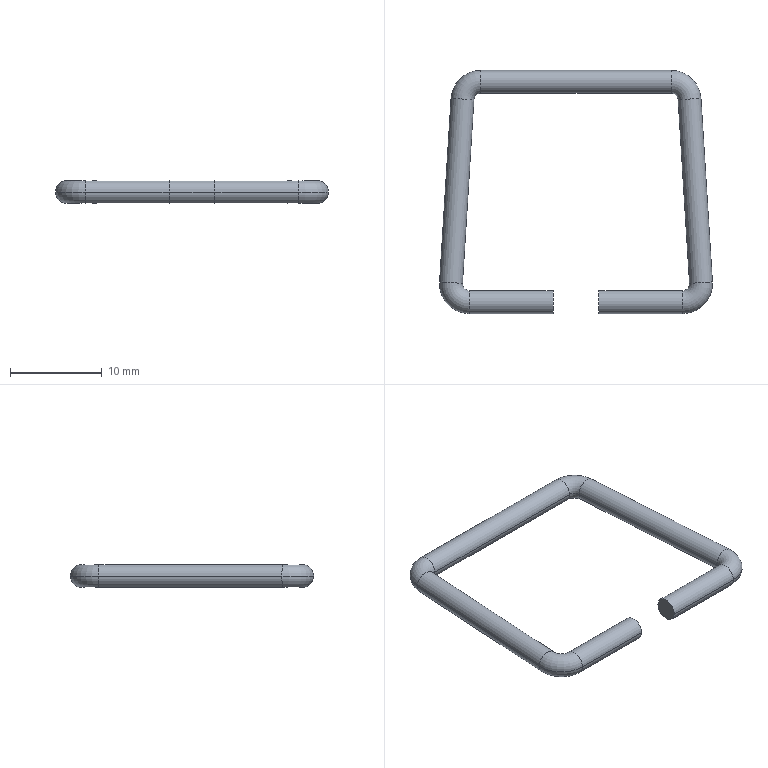Part | SolidWorks | features BaseBody 1 | 1 solid | 20 faces | box 29.742 x 26.5 x 2.5 mm | volume 449.782 mm3 | cylinder 10 | torus 8 | plane 2 | commonest cylinder face diameters 2.5 x10
STEP:
#1=CARTESIAN_POINT('',(11.621,1.25,0.));
#2=VERTEX_POINT('',#1);
#3=CARTESIAN_POINT('',(11.621,-1.25,0.));
#4=VERTEX_POINT('',#3);
#5=CARTESIAN_POINT('',(11.621,0.,0.));
#6=DIRECTION('',(1.,0.,0.));
#7=DIRECTION('',(0.,1.,0.));
#8=AXIS2_PLACEMENT_3D('',#5,#6,#7);
#9=CIRCLE('',#8,1.25);
#10=EDGE_CURVE('',#2,#4,#9,.T.);
#11=ORIENTED_EDGE('',*,*,#10,.T.);
#12=CARTESIAN_POINT('',(14.865,2.203,0.));
#13=VERTEX_POINT('',#12);
#14=CARTESIAN_POINT('',(11.621,2.,0.));
#15=DIRECTION('',(0.,0.,1.));
#16=DIRECTION('',(1.,0.,0.));
#17=AXIS2_PLACEMENT_3D('',#14,#15,#16);
#18=CIRCLE('',#17,3.25);
#19=EDGE_CURVE('',#4,#13,#18,.T.);
#20=ORIENTED_EDGE('',*,*,#19,.T.);
#21=CARTESIAN_POINT('',(12.37,2.047,0.));
#22=VERTEX_POINT('',#21);
#23=CARTESIAN_POINT('',(13.617,2.125,0.));
#24=DIRECTION('',(-0.06238,0.9981,0.));
#25=DIRECTION('',(0.9981,0.06238,0.));
#26=AXIS2_PLACEMENT_3D('',#23,#24,#25);
#27=CIRCLE('',#26,1.25);
#28=EDGE_CURVE('',#22,#13,#27,.T.);
#29=ORIENTED_EDGE('',*,*,#28,.F.);
#30=CARTESIAN_POINT('',(11.621,2.,0.));
#31=DIRECTION('',(0.,0.,1.));
#32=DIRECTION('',(1.,0.,0.));
#33=AXIS2_PLACEMENT_3D('',#30,#31,#32);
#34=CIRCLE('',#33,0.75);
#35=EDGE_CURVE('',#2,#22,#34,.T.);
#36=ORIENTED_EDGE('',*,*,#35,.F.);
#37=EDGE_LOOP('',(#11,#20,#29,#36));
#38=FACE_OUTER_BOUND('',#37,.T.);
#39=CARTESIAN_POINT('',(11.621,2.,0.));
#40=DIRECTION('',(0.,0.,1.));
#41=DIRECTION('',(0.,1.,0.));
#42=AXIS2_PLACEMENT_3D('',#39,#40,#41);
#43=TOROIDAL_SURFACE('',#42,2.,1.25);
#44=ADVANCED_FACE('',(#38),#43,.T.);
#45=CARTESIAN_POINT('',(11.12,22.047,0.));
#46=VERTEX_POINT('',#45);
#47=CARTESIAN_POINT('',(13.615,22.203,0.));
#48=VERTEX_POINT('',#47);
#49=CARTESIAN_POINT('',(12.367,22.125,0.));
#50=DIRECTION('',(-0.06238,0.9981,0.));
#51=DIRECTION('',(-0.9981,-0.06238,0.));
#52=AXIS2_PLACEMENT_3D('',#49,#50,#51);
#53=CIRCLE('',#52,1.25);
#54=EDGE_CURVE('',#46,#48,#53,.T.);
#55=ORIENTED_EDGE('',*,*,#54,.T.);
#56=CARTESIAN_POINT('',(10.371,25.25,0.));
#57=VERTEX_POINT('',#56);
#58=CARTESIAN_POINT('',(10.371,22.,0.));
#59=DIRECTION('',(0.,0.,1.));
#60=DIRECTION('',(1.,0.,0.));
#61=AXIS2_PLACEMENT_3D('',#58,#59,#60);
#62=CIRCLE('',#61,3.25);
#63=EDGE_CURVE('',#48,#57,#62,.T.);
#64=ORIENTED_EDGE('',*,*,#63,.T.);
#65=CARTESIAN_POINT('',(10.371,22.75,0.));
#66=VERTEX_POINT('',#65);
#67=CARTESIAN_POINT('',(10.371,24.,0.));
#68=DIRECTION('',(-1.,0.,0.));
#69=DIRECTION('',(0.,1.,0.));
#70=AXIS2_PLACEMENT_3D('',#67,#68,#69);
#71=CIRCLE('',#70,1.25);
#72=EDGE_CURVE('',#66,#57,#71,.T.);
#73=ORIENTED_EDGE('',*,*,#72,.F.);
#74=CARTESIAN_POINT('',(10.371,22.,0.));
#75=DIRECTION('',(0.,0.,1.));
#76=DIRECTION('',(1.,0.,0.));
#77=AXIS2_PLACEMENT_3D('',#74,#75,#76);
#78=CIRCLE('',#77,0.75);
#79=EDGE_CURVE('',#46,#66,#78,.T.);
#80=ORIENTED_EDGE('',*,*,#79,.F.);
#81=EDGE_LOOP('',(#55,#64,#73,#80));
#82=FACE_OUTER_BOUND('',#81,.T.);
#83=CARTESIAN_POINT('',(10.371,22.,0.));
#84=DIRECTION('',(0.,0.,1.));
#85=DIRECTION('',(-0.9981,-0.06238,0.));
#86=AXIS2_PLACEMENT_3D('',#83,#84,#85);
#87=TOROIDAL_SURFACE('',#86,2.,1.25);
#88=ADVANCED_FACE('',(#82),#87,.T.);
#89=CARTESIAN_POINT('',(-10.371,22.75,0.));
#90=VERTEX_POINT('',#89);
#91=CARTESIAN_POINT('',(-10.371,25.25,0.));
#92=VERTEX_POINT('',#91);
#93=CARTESIAN_POINT('',(-10.371,24.,0.));
#94=DIRECTION('',(-1.,0.,0.));
#95=DIRECTION('',(0.,-1.,0.));
#96=AXIS2_PLACEMENT_3D('',#93,#94,#95);
#97=CIRCLE('',#96,1.25);
#98=EDGE_CURVE('',#90,#92,#97,.T.);
#99=ORIENTED_EDGE('',*,*,#98,.T.);
#100=CARTESIAN_POINT('',(-13.615,22.203,0.));
#101=VERTEX_POINT('',#100);
#102=CARTESIAN_POINT('',(-10.371,22.,0.));
#103=DIRECTION('',(0.,0.,1.));
#104=DIRECTION('',(1.,0.,0.));
#105=AXIS2_PLACEMENT_3D('',#102,#103,#104);
#106=CIRCLE('',#105,3.25);
#107=EDGE_CURVE('',#92,#101,#106,.T.);
#108=ORIENTED_EDGE('',*,*,#107,.T.);
#109=CARTESIAN_POINT('',(-11.12,22.047,0.));
#110=VERTEX_POINT('',#109);
#111=CARTESIAN_POINT('',(-12.367,22.125,0.));
#112=DIRECTION('',(-0.06238,-0.9981,0.));
#113=DIRECTION('',(-0.9981,0.06238,0.));
#114=AXIS2_PLACEMENT_3D('',#111,#112,#113);
#115=CIRCLE('',#114,1.25);
#116=EDGE_CURVE('',#110,#101,#115,.T.);
#117=ORIENTED_EDGE('',*,*,#116,.F.);
#118=CARTESIAN_POINT('',(-10.371,22.,0.));
#119=DIRECTION('',(0.,0.,1.));
#120=DIRECTION('',(1.,0.,0.));
#121=AXIS2_PLACEMENT_3D('',#118,#119,#120);
#122=CIRCLE('',#121,0.75);
#123=EDGE_CURVE('',#90,#110,#122,.T.);
#124=ORIENTED_EDGE('',*,*,#123,.F.);
#125=EDGE_LOOP('',(#99,#108,#117,#124));
#126=FACE_OUTER_BOUND('',#125,.T.);
#127=CARTESIAN_POINT('',(-10.371,22.,0.));
#128=DIRECTION('',(0.,0.,1.));
#129=DIRECTION('',(0.,-1.,0.));
#130=AXIS2_PLACEMENT_3D('',#127,#128,#129);
#131=TOROIDAL_SURFACE('',#130,2.,1.25);
#132=ADVANCED_FACE('',(#126),#131,.T.);
#133=CARTESIAN_POINT('',(-12.37,2.047,0.));
#134=VERTEX_POINT('',#133);
#135=CARTESIAN_POINT('',(-14.865,2.203,0.));
#136=VERTEX_POINT('',#135);
#137=CARTESIAN_POINT('',(-13.617,2.125,0.));
#138=DIRECTION('',(-0.06238,-0.9981,0.));
#139=DIRECTION('',(0.9981,-0.06238,0.));
#140=AXIS2_PLACEMENT_3D('',#137,#138,#139);
#141=CIRCLE('',#140,1.25);
#142=EDGE_CURVE('',#134,#136,#141,.T.);
#143=ORIENTED_EDGE('',*,*,#142,.T.);
#144=CARTESIAN_POINT('',(-11.621,-1.25,0.));
#145=VERTEX_POINT('',#144);
#146=CARTESIAN_POINT('',(-11.621,2.,0.));
#147=DIRECTION('',(0.,0.,1.));
#148=DIRECTION('',(1.,0.,0.));
#149=AXIS2_PLACEMENT_3D('',#146,#147,#148);
#150=CIRCLE('',#149,3.25);
#151=EDGE_CURVE('',#136,#145,#150,.T.);
#152=ORIENTED_EDGE('',*,*,#151,.T.);
#153=CARTESIAN_POINT('',(-11.621,1.25,0.));
#154=VERTEX_POINT('',#153);
#155=CARTESIAN_POINT('',(-11.621,0.,0.));
#156=DIRECTION('',(1.,0.,0.));
#157=DIRECTION('',(0.,-1.,0.));
#158=AXIS2_PLACEMENT_3D('',#155,#156,#157);
#159=CIRCLE('',#158,1.25);
#160=EDGE_CURVE('',#154,#145,#159,.T.);
#161=ORIENTED_EDGE('',*,*,#160,.F.);
#162=CARTESIAN_POINT('',(-11.621,2.,0.));
#163=DIRECTION('',(0.,0.,1.));
#164=DIRECTION('',(1.,0.,0.));
#165=AXIS2_PLACEMENT_3D('',#162,#163,#164);
#166=CIRCLE('',#165,0.75);
#167=EDGE_CURVE('',#134,#154,#166,.T.);
#168=ORIENTED_EDGE('',*,*,#167,.F.);
#169=EDGE_LOOP('',(#143,#152,#161,#168));
#170=FACE_OUTER_BOUND('',#169,.T.);
#171=CARTESIAN_POINT('',(-11.621,2.,0.));
#172=DIRECTION('',(0.,0.,1.));
#173=DIRECTION('',(0.9981,-0.06238,0.));
#174=AXIS2_PLACEMENT_3D('',#171,#172,#173);
#175=TOROIDAL_SURFACE('',#174,2.,1.25);
#176=ADVANCED_FACE('',(#170),#175,.T.);
#177=CARTESIAN_POINT('',(2.5,1.25,0.));
#178=VERTEX_POINT('',#177);
#179=CARTESIAN_POINT('',(2.5,-1.25,0.));
#180=VERTEX_POINT('',#179);
#181=CARTESIAN_POINT('',(2.5,0.,0.));
#182=DIRECTION('',(1.,0.,0.));
#183=DIRECTION('',(0.,-1.,0.));
#184=AXIS2_PLACEMENT_3D('',#181,#182,#183);
#185=CIRCLE('',#184,1.25);
#186=EDGE_CURVE('',#178,#180,#185,.T.);
#187=ORIENTED_EDGE('',*,*,#186,.T.);
#188=CARTESIAN_POINT('',(2.5,-1.25,0.));
#189=DIRECTION('',(1.,0.,0.));
#190=VECTOR('',#189,1000.);
#191=LINE('',#188,#190);
#192=EDGE_CURVE('',#180,#4,#191,.T.);
#193=ORIENTED_EDGE('',*,*,#192,.T.);
#194=ORIENTED_EDGE('',*,*,#10,.F.);
#195=CARTESIAN_POINT('',(2.5,1.25,0.));
#196=DIRECTION('',(1.,0.,0.));
#197=VECTOR('',#196,1000.);
#198=LINE('',#195,#197);
#199=EDGE_CURVE('',#178,#2,#198,.T.);
#200=ORIENTED_EDGE('',*,*,#199,.F.);
#201=EDGE_LOOP('',(#187,#193,#194,#200));
#202=FACE_OUTER_BOUND('',#201,.T.);
#203=CARTESIAN_POINT('',(2.5,0.,0.));
#204=DIRECTION('',(1.,0.,0.));
#205=DIRECTION('',(0.,1.,0.));
#206=AXIS2_PLACEMENT_3D('',#203,#204,#205);
#207=CYLINDRICAL_SURFACE('',#206,1.25);
#208=ADVANCED_FACE('',(#202),#207,.T.);
#209=ORIENTED_EDGE('',*,*,#28,.T.);
#210=CARTESIAN_POINT('',(14.865,2.203,0.));
#211=DIRECTION('',(-0.06238,0.9981,0.));
#212=VECTOR('',#211,1000.);
#213=LINE('',#210,#212);
#214=EDGE_CURVE('',#13,#48,#213,.T.);
#215=ORIENTED_EDGE('',*,*,#214,.T.);
#216=ORIENTED_EDGE('',*,*,#54,.F.);
#217=CARTESIAN_POINT('',(12.37,2.047,0.));
#218=DIRECTION('',(-0.06238,0.9981,0.));
#219=VECTOR('',#218,1000.);
#220=LINE('',#217,#219);
#221=EDGE_CURVE('',#22,#46,#220,.T.);
#222=ORIENTED_EDGE('',*,*,#221,.F.);
#223=EDGE_LOOP('',(#209,#215,#216,#222));
#224=FACE_OUTER_BOUND('',#223,.T.);
#225=CARTESIAN_POINT('',(13.617,2.125,0.));
#226=DIRECTION('',(-0.06238,0.9981,0.));
#227=DIRECTION('',(-0.9981,-0.06238,0.));
#228=AXIS2_PLACEMENT_3D('',#225,#226,#227);
#229=CYLINDRICAL_SURFACE('',#228,1.25);
#230=ADVANCED_FACE('',(#224),#229,.T.);
#231=ORIENTED_EDGE('',*,*,#72,.T.);
#232=CARTESIAN_POINT('',(10.371,25.25,0.));
#233=DIRECTION('',(-1.,0.,0.));
#234=VECTOR('',#233,1000.);
#235=LINE('',#232,#234);
#236=EDGE_CURVE('',#57,#92,#235,.T.);
#237=ORIENTED_EDGE('',*,*,#236,.T.);
#238=ORIENTED_EDGE('',*,*,#98,.F.);
#239=CARTESIAN_POINT('',(10.371,22.75,0.));
#240=DIRECTION('',(-1.,0.,0.));
#241=VECTOR('',#240,1000.);
#242=LINE('',#239,#241);
#243=EDGE_CURVE('',#66,#90,#242,.T.);
#244=ORIENTED_EDGE('',*,*,#243,.F.);
#245=EDGE_LOOP('',(#231,#237,#238,#244));
#246=FACE_OUTER_BOUND('',#245,.T.);
#247=CARTESIAN_POINT('',(10.371,24.,0.));
#248=DIRECTION('',(-1.,0.,0.));
#249=DIRECTION('',(0.,-1.,0.));
#250=AXIS2_PLACEMENT_3D('',#247,#248,#249);
#251=CYLINDRICAL_SURFACE('',#250,1.25);
#252=ADVANCED_FACE('',(#246),#251,.T.);
#253=ORIENTED_EDGE('',*,*,#116,.T.);
#254=CARTESIAN_POINT('',(-13.615,22.203,0.));
#255=DIRECTION('',(-0.06238,-0.9981,0.));
#256=VECTOR('',#255,1000.);
#257=LINE('',#254,#256);
#258=EDGE_CURVE('',#101,#136,#257,.T.);
#259=ORIENTED_EDGE('',*,*,#258,.T.);
#260=ORIENTED_EDGE('',*,*,#142,.F.);
#261=CARTESIAN_POINT('',(-11.12,22.047,0.));
#262=DIRECTION('',(-0.06238,-0.9981,0.));
#263=VECTOR('',#262,1000.);
#264=LINE('',#261,#263);
#265=EDGE_CURVE('',#110,#134,#264,.T.);
#266=ORIENTED_EDGE('',*,*,#265,.F.);
#267=EDGE_LOOP('',(#253,#259,#260,#266));
#268=FACE_OUTER_BOUND('',#267,.T.);
#269=CARTESIAN_POINT('',(-12.367,22.125,0.));
#270=DIRECTION('',(-0.06238,-0.9981,0.));
#271=DIRECTION('',(0.9981,-0.06238,0.));
#272=AXIS2_PLACEMENT_3D('',#269,#270,#271);
#273=CYLINDRICAL_SURFACE('',#272,1.25);
#274=ADVANCED_FACE('',(#268),#273,.T.);
#275=ORIENTED_EDGE('',*,*,#160,.T.);
#276=CARTESIAN_POINT('',(-2.5,-1.25,0.));
#277=VERTEX_POINT('',#276);
#278=CARTESIAN_POINT('',(-11.621,-1.25,0.));
#279=DIRECTION('',(1.,0.,0.));
#280=VECTOR('',#279,1000.);
#281=LINE('',#278,#280);
#282=EDGE_CURVE('',#145,#277,#281,.T.);
#283=ORIENTED_EDGE('',*,*,#282,.T.);
#284=CARTESIAN_POINT('',(-2.5,1.25,0.));
#285=VERTEX_POINT('',#284);
#286=CARTESIAN_POINT('',(-2.5,0.,0.));
#287=DIRECTION('',(1.,0.,0.));
#288=DIRECTION('',(0.,1.,0.));
#289=AXIS2_PLACEMENT_3D('',#286,#287,#288);
#290=CIRCLE('',#289,1.25);
#291=EDGE_CURVE('',#285,#277,#290,.T.);
#292=ORIENTED_EDGE('',*,*,#291,.F.);
#293=CARTESIAN_POINT('',(-11.621,1.25,0.));
#294=DIRECTION('',(1.,0.,0.));
#295=VECTOR('',#294,1000.);
#296=LINE('',#293,#295);
#297=EDGE_CURVE('',#154,#285,#296,.T.);
#298=ORIENTED_EDGE('',*,*,#297,.F.);
#299=EDGE_LOOP('',(#275,#283,#292,#298));
#300=FACE_OUTER_BOUND('',#299,.T.);
#301=CARTESIAN_POINT('',(-11.621,0.,0.));
#302=DIRECTION('',(1.,0.,0.));
#303=DIRECTION('',(0.,1.,0.));
#304=AXIS2_PLACEMENT_3D('',#301,#302,#303);
#305=CYLINDRICAL_SURFACE('',#304,1.25);
#306=ADVANCED_FACE('',(#300),#305,.T.);
#307=ORIENTED_EDGE('',*,*,#291,.T.);
#308=CARTESIAN_POINT('',(-2.5,0.,0.));
#309=DIRECTION('',(1.,0.,0.));
#310=DIRECTION('',(0.,1.,0.));
#311=AXIS2_PLACEMENT_3D('',#308,#309,#310);
#312=CIRCLE('',#311,1.25);
#313=EDGE_CURVE('',#277,#285,#312,.T.);
#314=ORIENTED_EDGE('',*,*,#313,.T.);
#315=EDGE_LOOP('',(#307,#314));
#316=FACE_OUTER_BOUND('',#315,.T.);
#317=CARTESIAN_POINT('',(-2.5,0.,0.));
#318=DIRECTION('',(1.,0.,0.));
#319=DIRECTION('',(0.,1.,0.));
#320=AXIS2_PLACEMENT_3D('',#317,#318,#319);
#321=PLANE('',#320);
#322=ADVANCED_FACE('',(#316),#321,.T.);
#323=ORIENTED_EDGE('',*,*,#282,.F.);
#324=CARTESIAN_POINT('',(-11.621,0.,0.));
#325=DIRECTION('',(1.,0.,0.));
#326=DIRECTION('',(0.,-1.,0.));
#327=AXIS2_PLACEMENT_3D('',#324,#325,#326);
#328=CIRCLE('',#327,1.25);
#329=EDGE_CURVE('',#145,#154,#328,.T.);
#330=ORIENTED_EDGE('',*,*,#329,.T.);
#331=ORIENTED_EDGE('',*,*,#297,.T.);
#332=ORIENTED_EDGE('',*,*,#313,.F.);
#333=EDGE_LOOP('',(#323,#330,#331,#332));
#334=FACE_OUTER_BOUND('',#333,.T.);
#335=CARTESIAN_POINT('',(-11.621,0.,0.));
#336=DIRECTION('',(1.,0.,0.));
#337=DIRECTION('',(0.,1.,0.));
#338=AXIS2_PLACEMENT_3D('',#335,#336,#337);
#339=CYLINDRICAL_SURFACE('',#338,1.25);
#340=ADVANCED_FACE('',(#334),#339,.T.);
#341=ORIENTED_EDGE('',*,*,#151,.F.);
#342=CARTESIAN_POINT('',(-13.617,2.125,0.));
#343=DIRECTION('',(-0.06238,-0.9981,0.));
#344=DIRECTION('',(0.9981,-0.06238,0.));
#345=AXIS2_PLACEMENT_3D('',#342,#343,#344);
#346=CIRCLE('',#345,1.25);
#347=EDGE_CURVE('',#136,#134,#346,.T.);
#348=ORIENTED_EDGE('',*,*,#347,.T.);
#349=ORIENTED_EDGE('',*,*,#167,.T.);
#350=ORIENTED_EDGE('',*,*,#329,.F.);
#351=EDGE_LOOP('',(#341,#348,#349,#350));
#352=FACE_OUTER_BOUND('',#351,.T.);
#353=CARTESIAN_POINT('',(-11.621,2.,0.));
#354=DIRECTION('',(0.,0.,1.));
#355=DIRECTION('',(0.9981,-0.06238,0.));
#356=AXIS2_PLACEMENT_3D('',#353,#354,#355);
#357=TOROIDAL_SURFACE('',#356,2.,1.25);
#358=ADVANCED_FACE('',(#352),#357,.T.);
#359=ORIENTED_EDGE('',*,*,#258,.F.);
#360=CARTESIAN_POINT('',(-12.367,22.125,0.));
#361=DIRECTION('',(-0.06238,-0.9981,0.));
#362=DIRECTION('',(-0.9981,0.06238,0.));
#363=AXIS2_PLACEMENT_3D('',#360,#361,#362);
#364=CIRCLE('',#363,1.25);
#365=EDGE_CURVE('',#101,#110,#364,.T.);
#366=ORIENTED_EDGE('',*,*,#365,.T.);
#367=ORIENTED_EDGE('',*,*,#265,.T.);
#368=ORIENTED_EDGE('',*,*,#347,.F.);
#369=EDGE_LOOP('',(#359,#366,#367,#368));
#370=FACE_OUTER_BOUND('',#369,.T.);
#371=CARTESIAN_POINT('',(-12.367,22.125,0.));
#372=DIRECTION('',(-0.06238,-0.9981,0.));
#373=DIRECTION('',(0.9981,-0.06238,0.));
#374=AXIS2_PLACEMENT_3D('',#371,#372,#373);
#375=CYLINDRICAL_SURFACE('',#374,1.25);
#376=ADVANCED_FACE('',(#370),#375,.T.);
#377=ORIENTED_EDGE('',*,*,#107,.F.);
#378=CARTESIAN_POINT('',(-10.371,24.,0.));
#379=DIRECTION('',(-1.,0.,0.));
#380=DIRECTION('',(0.,-1.,0.));
#381=AXIS2_PLACEMENT_3D('',#378,#379,#380);
#382=CIRCLE('',#381,1.25);
#383=EDGE_CURVE('',#92,#90,#382,.T.);
#384=ORIENTED_EDGE('',*,*,#383,.T.);
#385=ORIENTED_EDGE('',*,*,#123,.T.);
#386=ORIENTED_EDGE('',*,*,#365,.F.);
#387=EDGE_LOOP('',(#377,#384,#385,#386));
#388=FACE_OUTER_BOUND('',#387,.T.);
#389=CARTESIAN_POINT('',(-10.371,22.,0.));
#390=DIRECTION('',(0.,0.,1.));
#391=DIRECTION('',(0.,-1.,0.));
#392=AXIS2_PLACEMENT_3D('',#389,#390,#391);
#393=TOROIDAL_SURFACE('',#392,2.,1.25);
#394=ADVANCED_FACE('',(#388),#393,.T.);
#395=ORIENTED_EDGE('',*,*,#236,.F.);
#396=CARTESIAN_POINT('',(10.371,24.,0.));
#397=DIRECTION('',(-1.,0.,0.));
#398=DIRECTION('',(0.,1.,0.));
#399=AXIS2_PLACEMENT_3D('',#396,#397,#398);
#400=CIRCLE('',#399,1.25);
#401=EDGE_CURVE('',#57,#66,#400,.T.);
#402=ORIENTED_EDGE('',*,*,#401,.T.);
#403=ORIENTED_EDGE('',*,*,#243,.T.);
#404=ORIENTED_EDGE('',*,*,#383,.F.);
#405=EDGE_LOOP('',(#395,#402,#403,#404));
#406=FACE_OUTER_BOUND('',#405,.T.);
#407=CARTESIAN_POINT('',(10.371,24.,0.));
#408=DIRECTION('',(-1.,0.,0.));
#409=DIRECTION('',(0.,-1.,0.));
#410=AXIS2_PLACEMENT_3D('',#407,#408,#409);
#411=CYLINDRICAL_SURFACE('',#410,1.25);
#412=ADVANCED_FACE('',(#406),#411,.T.);
#413=ORIENTED_EDGE('',*,*,#63,.F.);
#414=CARTESIAN_POINT('',(12.367,22.125,0.));
#415=DIRECTION('',(-0.06238,0.9981,0.));
#416=DIRECTION('',(-0.9981,-0.06238,0.));
#417=AXIS2_PLACEMENT_3D('',#414,#415,#416);
#418=CIRCLE('',#417,1.25);
#419=EDGE_CURVE('',#48,#46,#418,.T.);
#420=ORIENTED_EDGE('',*,*,#419,.T.);
#421=ORIENTED_EDGE('',*,*,#79,.T.);
#422=ORIENTED_EDGE('',*,*,#401,.F.);
#423=EDGE_LOOP('',(#413,#420,#421,#422));
#424=FACE_OUTER_BOUND('',#423,.T.);
#425=CARTESIAN_POINT('',(10.371,22.,0.));
#426=DIRECTION('',(0.,0.,1.));
#427=DIRECTION('',(-0.9981,-0.06238,0.));
#428=AXIS2_PLACEMENT_3D('',#425,#426,#427);
#429=TOROIDAL_SURFACE('',#428,2.,1.25);
#430=ADVANCED_FACE('',(#424),#429,.T.);
#431=ORIENTED_EDGE('',*,*,#214,.F.);
#432=CARTESIAN_POINT('',(13.617,2.125,0.));
#433=DIRECTION('',(-0.06238,0.9981,0.));
#434=DIRECTION('',(0.9981,0.06238,0.));
#435=AXIS2_PLACEMENT_3D('',#432,#433,#434);
#436=CIRCLE('',#435,1.25);
#437=EDGE_CURVE('',#13,#22,#436,.T.);
#438=ORIENTED_EDGE('',*,*,#437,.T.);
#439=ORIENTED_EDGE('',*,*,#221,.T.);
#440=ORIENTED_EDGE('',*,*,#419,.F.);
#441=EDGE_LOOP('',(#431,#438,#439,#440));
#442=FACE_OUTER_BOUND('',#441,.T.);
#443=CARTESIAN_POINT('',(13.617,2.125,0.));
#444=DIRECTION('',(-0.06238,0.9981,0.));
#445=DIRECTION('',(-0.9981,-0.06238,0.));
#446=AXIS2_PLACEMENT_3D('',#443,#444,#445);
#447=CYLINDRICAL_SURFACE('',#446,1.25);
#448=ADVANCED_FACE('',(#442),#447,.T.);
#449=ORIENTED_EDGE('',*,*,#19,.F.);
#450=CARTESIAN_POINT('',(11.621,0.,0.));
#451=DIRECTION('',(1.,0.,0.));
#452=DIRECTION('',(0.,1.,0.));
#453=AXIS2_PLACEMENT_3D('',#450,#451,#452);
#454=CIRCLE('',#453,1.25);
#455=EDGE_CURVE('',#4,#2,#454,.T.);
#456=ORIENTED_EDGE('',*,*,#455,.T.);
#457=ORIENTED_EDGE('',*,*,#35,.T.);
#458=ORIENTED_EDGE('',*,*,#437,.F.);
#459=EDGE_LOOP('',(#449,#456,#457,#458));
#460=FACE_OUTER_BOUND('',#459,.T.);
#461=CARTESIAN_POINT('',(11.621,2.,0.));
#462=DIRECTION('',(0.,0.,1.));
#463=DIRECTION('',(0.,1.,0.));
#464=AXIS2_PLACEMENT_3D('',#461,#462,#463);
#465=TOROIDAL_SURFACE('',#464,2.,1.25);
#466=ADVANCED_FACE('',(#460),#465,.T.);
#467=ORIENTED_EDGE('',*,*,#192,.F.);
#468=CARTESIAN_POINT('',(2.5,0.,0.));
#469=DIRECTION('',(1.,0.,0.));
#470=DIRECTION('',(0.,-1.,0.));
#471=AXIS2_PLACEMENT_3D('',#468,#469,#470);
#472=CIRCLE('',#471,1.25);
#473=EDGE_CURVE('',#180,#178,#472,.T.);
#474=ORIENTED_EDGE('',*,*,#473,.T.);
#475=ORIENTED_EDGE('',*,*,#199,.T.);
#476=ORIENTED_EDGE('',*,*,#455,.F.);
#477=EDGE_LOOP('',(#467,#474,#475,#476));
#478=FACE_OUTER_BOUND('',#477,.T.);
#479=CARTESIAN_POINT('',(2.5,0.,0.));
#480=DIRECTION('',(1.,0.,0.));
#481=DIRECTION('',(0.,1.,0.));
#482=AXIS2_PLACEMENT_3D('',#479,#480,#481);
#483=CYLINDRICAL_SURFACE('',#482,1.25);
#484=ADVANCED_FACE('',(#478),#483,.T.);
#485=ORIENTED_EDGE('',*,*,#186,.F.);
#486=ORIENTED_EDGE('',*,*,#473,.F.);
#487=EDGE_LOOP('',(#485,#486));
#488=FACE_OUTER_BOUND('',#487,.T.);
#489=CARTESIAN_POINT('',(2.5,0.,0.));
#490=DIRECTION('',(1.,0.,0.));
#491=DIRECTION('',(0.,1.,0.));
#492=AXIS2_PLACEMENT_3D('',#489,#490,#491);
#493=PLANE('',#492);
#494=ADVANCED_FACE('',(#488),#493,.F.);
#495=CLOSED_SHELL('',(#44,#88,#132,#176,#208,#230,#252,#274,#306,#322,#340,#358,#376,#394,#412,#430,#448,#466,#484,#494));
#496=MANIFOLD_SOLID_BREP('',#495);
#497=CARTESIAN_POINT('',(0.,0.,0.));
#498=DIRECTION('',(0.,0.,1.));
#499=DIRECTION('',(1.,0.,0.));
#500=AXIS2_PLACEMENT_3D('',#497,#498,#499);
#501=(LENGTH_UNIT()NAMED_UNIT(*)SI_UNIT(.MILLI.,.METRE.));
#502=UNCERTAINTY_MEASURE_WITH_UNIT(LENGTH_MEASURE(0.00001),#501,'','');
#503=(NAMED_UNIT(*)PLANE_ANGLE_UNIT()SI_UNIT($,.RADIAN.));
#504=(NAMED_UNIT(*)SI_UNIT($,.STERADIAN.)SOLID_ANGLE_UNIT());
#505=(GEOMETRIC_REPRESENTATION_CONTEXT(3)GLOBAL_UNCERTAINTY_ASSIGNED_CONTEXT((#502))GLOBAL_UNIT_ASSIGNED_CONTEXT((#501,#503,#504))REPRESENTATION_CONTEXT('',''));
#506=ADVANCED_BREP_SHAPE_REPRESENTATION('',(#496,#500),#505);